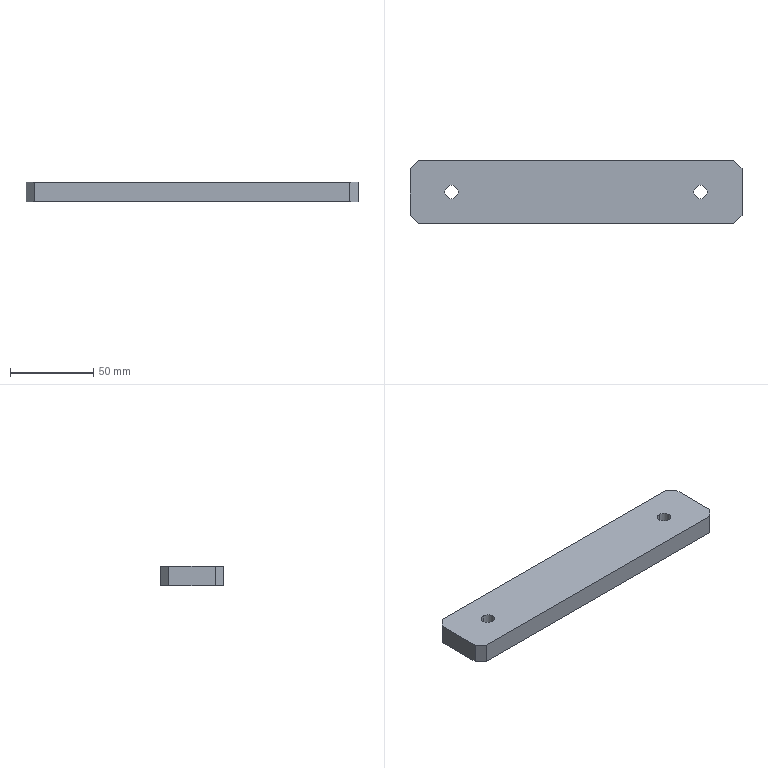Part | STEP file | [13] | 1 solid | 14 faces | box 200 x 38 x 12 mm | volume 89394 mm3 | plane 10 | cylinder 4 | commonest cylinder face diameters 8 x4
STEP:
#1=CARTESIAN_POINT('',(0.,0.,0.));
#2=DIRECTION('',(0.,0.,1.));
#3=DIRECTION('',(1.,0.,0.));
#4=AXIS2_PLACEMENT_3D('',#1,#2,#3);
#5=CARTESIAN_POINT('',(25.,23.,-3.));
#6=VERTEX_POINT('',#5);
#7=CARTESIAN_POINT('',(25.,23.,9.));
#8=VERTEX_POINT('',#7);
#9=CARTESIAN_POINT('',(25.,23.,-3.));
#10=DIRECTION('',(0.,0.,1.));
#11=VECTOR('',#10,1.);
#12=LINE('',#9,#11);
#13=CARTESIAN_POINT('',(25.,19.,-3.));
#14=DIRECTION('',(0.,0.,1.));
#15=DIRECTION('',(0.,1.,0.));
#16=AXIS2_PLACEMENT_3D('',#13,#14,#15);
#17=CYLINDRICAL_SURFACE('',#16,4.);
#18=CARTESIAN_POINT('',(6.283,0.));
#19=DIRECTION('',(0.,1.));
#20=VECTOR('',#19,1.);
#21=LINE('',#18,#20);
#22=(GEOMETRIC_REPRESENTATION_CONTEXT(2)PARAMETRIC_REPRESENTATION_CONTEXT()REPRESENTATION_CONTEXT('',''));
#23=DEFINITIONAL_REPRESENTATION('',(#21),#22);
#24=PCURVE('',#17,#23);
#25=CARTESIAN_POINT('',(25.,19.,-3.));
#26=DIRECTION('',(0.,0.,1.));
#27=DIRECTION('',(0.,1.,0.));
#28=AXIS2_PLACEMENT_3D('',#25,#26,#27);
#29=CYLINDRICAL_SURFACE('',#28,4.);
#30=CARTESIAN_POINT('',(0.,0.));
#31=DIRECTION('',(0.,1.));
#32=VECTOR('',#31,1.);
#33=LINE('',#30,#32);
#34=(GEOMETRIC_REPRESENTATION_CONTEXT(2)PARAMETRIC_REPRESENTATION_CONTEXT()REPRESENTATION_CONTEXT('',''));
#35=DEFINITIONAL_REPRESENTATION('',(#33),#34);
#36=PCURVE('',#29,#35);
#37=SURFACE_CURVE('',#12,(#24,#36),.PCURVE_S1.);
#38=EDGE_CURVE('',#6,#8,#37,.T.);
#39=ORIENTED_EDGE('',*,*,#38,.T.);
#40=CARTESIAN_POINT('',(25.,15.,9.));
#41=VERTEX_POINT('',#40);
#42=CARTESIAN_POINT('',(25.,19.,9.));
#43=DIRECTION('',(0.,0.,-1.));
#44=DIRECTION('',(0.,-1.,0.));
#45=AXIS2_PLACEMENT_3D('',#42,#43,#44);
#46=CIRCLE('',#45,4.);
#47=CARTESIAN_POINT('',(9.425,12.));
#48=DIRECTION('',(-1.,0.));
#49=VECTOR('',#48,1.);
#50=LINE('',#47,#49);
#51=(GEOMETRIC_REPRESENTATION_CONTEXT(2)PARAMETRIC_REPRESENTATION_CONTEXT()REPRESENTATION_CONTEXT('',''));
#52=DEFINITIONAL_REPRESENTATION('',(#50),#51);
#53=PCURVE('',#17,#52);
#54=CARTESIAN_POINT('',(100.,19.,9.));
#55=DIRECTION('',(0.,0.,1.));
#56=DIRECTION('',(0.,1.,0.));
#57=AXIS2_PLACEMENT_3D('',#54,#55,#56);
#58=PLANE('',#57);
#59=CARTESIAN_POINT('',(-4.,75.));
#60=CARTESIAN_POINT('',(-4.,81.928));
#61=CARTESIAN_POINT('',(2.,78.464));
#62=CARTESIAN_POINT('',(8.,75.));
#63=CARTESIAN_POINT('',(2.,71.536));
#64=CARTESIAN_POINT('',(-4.,68.072));
#65=CARTESIAN_POINT('',(-4.,75.));
#66=(BOUNDED_CURVE()B_SPLINE_CURVE(2,(#59,#60,#61,#62,#63,#64,#65),.UNSPECIFIED.,.T.,.F.)B_SPLINE_CURVE_WITH_KNOTS((1,2,2,2,2,1),(-2.094,0.,2.094,4.189,6.283,8.378),.UNSPECIFIED.)CURVE()GEOMETRIC_REPRESENTATION_ITEM()RATIONAL_B_SPLINE_CURVE((1.,0.5,1.,0.5,1.,0.5,1.))REPRESENTATION_ITEM(''));
#67=(GEOMETRIC_REPRESENTATION_CONTEXT(2)PARAMETRIC_REPRESENTATION_CONTEXT()REPRESENTATION_CONTEXT('',''));
#68=DEFINITIONAL_REPRESENTATION('',(#66),#67);
#69=PCURVE('',#58,#68);
#70=SURFACE_CURVE('',#46,(#53,#69),.PCURVE_S1.);
#71=EDGE_CURVE('',#8,#41,#70,.T.);
#72=ORIENTED_EDGE('',*,*,#71,.T.);
#73=CARTESIAN_POINT('',(25.,15.,-3.));
#74=VERTEX_POINT('',#73);
#75=CARTESIAN_POINT('',(25.,15.,-3.));
#76=DIRECTION('',(0.,0.,1.));
#77=VECTOR('',#76,1.);
#78=LINE('',#75,#77);
#79=CARTESIAN_POINT('',(3.142,0.));
#80=DIRECTION('',(0.,1.));
#81=VECTOR('',#80,1.);
#82=LINE('',#79,#81);
#83=(GEOMETRIC_REPRESENTATION_CONTEXT(2)PARAMETRIC_REPRESENTATION_CONTEXT()REPRESENTATION_CONTEXT('',''));
#84=DEFINITIONAL_REPRESENTATION('',(#82),#83);
#85=PCURVE('',#17,#84);
#86=CARTESIAN_POINT('',(3.142,0.));
#87=DIRECTION('',(0.,1.));
#88=VECTOR('',#87,1.);
#89=LINE('',#86,#88);
#90=(GEOMETRIC_REPRESENTATION_CONTEXT(2)PARAMETRIC_REPRESENTATION_CONTEXT()REPRESENTATION_CONTEXT('',''));
#91=DEFINITIONAL_REPRESENTATION('',(#89),#90);
#92=PCURVE('',#29,#91);
#93=SURFACE_CURVE('',#78,(#85,#92),.PCURVE_S1.);
#94=EDGE_CURVE('',#74,#41,#93,.T.);
#95=ORIENTED_EDGE('',*,*,#94,.F.);
#96=CARTESIAN_POINT('',(25.,19.,-3.));
#97=DIRECTION('',(0.,0.,1.));
#98=DIRECTION('',(0.,1.,0.));
#99=AXIS2_PLACEMENT_3D('',#96,#97,#98);
#100=CIRCLE('',#99,4.);
#101=CARTESIAN_POINT('',(0.,0.));
#102=DIRECTION('',(1.,0.));
#103=VECTOR('',#102,1.);
#104=LINE('',#101,#103);
#105=(GEOMETRIC_REPRESENTATION_CONTEXT(2)PARAMETRIC_REPRESENTATION_CONTEXT()REPRESENTATION_CONTEXT('',''));
#106=DEFINITIONAL_REPRESENTATION('',(#104),#105);
#107=PCURVE('',#17,#106);
#108=CARTESIAN_POINT('',(100.,19.,-3.));
#109=DIRECTION('',(0.,0.,-1.));
#110=DIRECTION('',(0.,-1.,0.));
#111=AXIS2_PLACEMENT_3D('',#108,#109,#110);
#112=PLANE('',#111);
#113=CARTESIAN_POINT('',(-4.,75.));
#114=CARTESIAN_POINT('',(-4.,81.928));
#115=CARTESIAN_POINT('',(2.,78.464));
#116=CARTESIAN_POINT('',(8.,75.));
#117=CARTESIAN_POINT('',(2.,71.536));
#118=CARTESIAN_POINT('',(-4.,68.072));
#119=CARTESIAN_POINT('',(-4.,75.));
#120=(BOUNDED_CURVE()B_SPLINE_CURVE(2,(#113,#114,#115,#116,#117,#118,#119),.UNSPECIFIED.,.T.,.F.)B_SPLINE_CURVE_WITH_KNOTS((1,2,2,2,2,1),(-2.094,0.,2.094,4.189,6.283,8.378),.UNSPECIFIED.)CURVE()GEOMETRIC_REPRESENTATION_ITEM()RATIONAL_B_SPLINE_CURVE((1.,0.5,1.,0.5,1.,0.5,1.))REPRESENTATION_ITEM(''));
#121=(GEOMETRIC_REPRESENTATION_CONTEXT(2)PARAMETRIC_REPRESENTATION_CONTEXT()REPRESENTATION_CONTEXT('',''));
#122=DEFINITIONAL_REPRESENTATION('',(#120),#121);
#123=PCURVE('',#112,#122);
#124=SURFACE_CURVE('',#100,(#107,#123),.PCURVE_S1.);
#125=EDGE_CURVE('',#74,#6,#124,.T.);
#126=ORIENTED_EDGE('',*,*,#125,.T.);
#127=EDGE_LOOP('',(#39,#72,#95,#126));
#128=FACE_BOUND('',#127,.F.);
#129=ADVANCED_FACE('',(#128),#17,.F.);
#130=CARTESIAN_POINT('',(175.,23.,-3.));
#131=VERTEX_POINT('',#130);
#132=CARTESIAN_POINT('',(175.,23.,9.));
#133=VERTEX_POINT('',#132);
#134=CARTESIAN_POINT('',(175.,23.,-3.));
#135=DIRECTION('',(0.,0.,1.));
#136=VECTOR('',#135,1.);
#137=LINE('',#134,#136);
#138=CARTESIAN_POINT('',(175.,19.,-3.));
#139=DIRECTION('',(0.,0.,1.));
#140=DIRECTION('',(0.,1.,0.));
#141=AXIS2_PLACEMENT_3D('',#138,#139,#140);
#142=CYLINDRICAL_SURFACE('',#141,4.);
#143=CARTESIAN_POINT('',(6.283,0.));
#144=DIRECTION('',(0.,1.));
#145=VECTOR('',#144,1.);
#146=LINE('',#143,#145);
#147=(GEOMETRIC_REPRESENTATION_CONTEXT(2)PARAMETRIC_REPRESENTATION_CONTEXT()REPRESENTATION_CONTEXT('',''));
#148=DEFINITIONAL_REPRESENTATION('',(#146),#147);
#149=PCURVE('',#142,#148);
#150=CARTESIAN_POINT('',(175.,19.,-3.));
#151=DIRECTION('',(0.,0.,1.));
#152=DIRECTION('',(0.,1.,0.));
#153=AXIS2_PLACEMENT_3D('',#150,#151,#152);
#154=CYLINDRICAL_SURFACE('',#153,4.);
#155=CARTESIAN_POINT('',(0.,0.));
#156=DIRECTION('',(0.,1.));
#157=VECTOR('',#156,1.);
#158=LINE('',#155,#157);
#159=(GEOMETRIC_REPRESENTATION_CONTEXT(2)PARAMETRIC_REPRESENTATION_CONTEXT()REPRESENTATION_CONTEXT('',''));
#160=DEFINITIONAL_REPRESENTATION('',(#158),#159);
#161=PCURVE('',#154,#160);
#162=SURFACE_CURVE('',#137,(#149,#161),.PCURVE_S1.);
#163=EDGE_CURVE('',#131,#133,#162,.T.);
#164=ORIENTED_EDGE('',*,*,#163,.T.);
#165=CARTESIAN_POINT('',(175.,15.,9.));
#166=VERTEX_POINT('',#165);
#167=CARTESIAN_POINT('',(175.,19.,9.));
#168=DIRECTION('',(0.,0.,-1.));
#169=DIRECTION('',(0.,-1.,0.));
#170=AXIS2_PLACEMENT_3D('',#167,#168,#169);
#171=CIRCLE('',#170,4.);
#172=CARTESIAN_POINT('',(9.425,12.));
#173=DIRECTION('',(-1.,0.));
#174=VECTOR('',#173,1.);
#175=LINE('',#172,#174);
#176=(GEOMETRIC_REPRESENTATION_CONTEXT(2)PARAMETRIC_REPRESENTATION_CONTEXT()REPRESENTATION_CONTEXT('',''));
#177=DEFINITIONAL_REPRESENTATION('',(#175),#176);
#178=PCURVE('',#142,#177);
#179=CARTESIAN_POINT('',(-4.,-75.));
#180=CARTESIAN_POINT('',(-4.,-68.072));
#181=CARTESIAN_POINT('',(2.,-71.536));
#182=CARTESIAN_POINT('',(8.,-75.));
#183=CARTESIAN_POINT('',(2.,-78.464));
#184=CARTESIAN_POINT('',(-4.,-81.928));
#185=CARTESIAN_POINT('',(-4.,-75.));
#186=(BOUNDED_CURVE()B_SPLINE_CURVE(2,(#179,#180,#181,#182,#183,#184,#185),.UNSPECIFIED.,.T.,.F.)B_SPLINE_CURVE_WITH_KNOTS((1,2,2,2,2,1),(-2.094,0.,2.094,4.189,6.283,8.378),.UNSPECIFIED.)CURVE()GEOMETRIC_REPRESENTATION_ITEM()RATIONAL_B_SPLINE_CURVE((1.,0.5,1.,0.5,1.,0.5,1.))REPRESENTATION_ITEM(''));
#187=(GEOMETRIC_REPRESENTATION_CONTEXT(2)PARAMETRIC_REPRESENTATION_CONTEXT()REPRESENTATION_CONTEXT('',''));
#188=DEFINITIONAL_REPRESENTATION('',(#186),#187);
#189=PCURVE('',#58,#188);
#190=SURFACE_CURVE('',#171,(#178,#189),.PCURVE_S1.);
#191=EDGE_CURVE('',#133,#166,#190,.T.);
#192=ORIENTED_EDGE('',*,*,#191,.T.);
#193=CARTESIAN_POINT('',(175.,15.,-3.));
#194=VERTEX_POINT('',#193);
#195=CARTESIAN_POINT('',(175.,15.,-3.));
#196=DIRECTION('',(0.,0.,1.));
#197=VECTOR('',#196,1.);
#198=LINE('',#195,#197);
#199=CARTESIAN_POINT('',(3.142,0.));
#200=DIRECTION('',(0.,1.));
#201=VECTOR('',#200,1.);
#202=LINE('',#199,#201);
#203=(GEOMETRIC_REPRESENTATION_CONTEXT(2)PARAMETRIC_REPRESENTATION_CONTEXT()REPRESENTATION_CONTEXT('',''));
#204=DEFINITIONAL_REPRESENTATION('',(#202),#203);
#205=PCURVE('',#142,#204);
#206=CARTESIAN_POINT('',(3.142,0.));
#207=DIRECTION('',(0.,1.));
#208=VECTOR('',#207,1.);
#209=LINE('',#206,#208);
#210=(GEOMETRIC_REPRESENTATION_CONTEXT(2)PARAMETRIC_REPRESENTATION_CONTEXT()REPRESENTATION_CONTEXT('',''));
#211=DEFINITIONAL_REPRESENTATION('',(#209),#210);
#212=PCURVE('',#154,#211);
#213=SURFACE_CURVE('',#198,(#205,#212),.PCURVE_S1.);
#214=EDGE_CURVE('',#194,#166,#213,.T.);
#215=ORIENTED_EDGE('',*,*,#214,.F.);
#216=CARTESIAN_POINT('',(175.,19.,-3.));
#217=DIRECTION('',(0.,0.,1.));
#218=DIRECTION('',(0.,1.,0.));
#219=AXIS2_PLACEMENT_3D('',#216,#217,#218);
#220=CIRCLE('',#219,4.);
#221=CARTESIAN_POINT('',(0.,0.));
#222=DIRECTION('',(1.,0.));
#223=VECTOR('',#222,1.);
#224=LINE('',#221,#223);
#225=(GEOMETRIC_REPRESENTATION_CONTEXT(2)PARAMETRIC_REPRESENTATION_CONTEXT()REPRESENTATION_CONTEXT('',''));
#226=DEFINITIONAL_REPRESENTATION('',(#224),#225);
#227=PCURVE('',#142,#226);
#228=CARTESIAN_POINT('',(-4.,-75.));
#229=CARTESIAN_POINT('',(-4.,-68.072));
#230=CARTESIAN_POINT('',(2.,-71.536));
#231=CARTESIAN_POINT('',(8.,-75.));
#232=CARTESIAN_POINT('',(2.,-78.464));
#233=CARTESIAN_POINT('',(-4.,-81.928));
#234=CARTESIAN_POINT('',(-4.,-75.));
#235=(BOUNDED_CURVE()B_SPLINE_CURVE(2,(#228,#229,#230,#231,#232,#233,#234),.UNSPECIFIED.,.T.,.F.)B_SPLINE_CURVE_WITH_KNOTS((1,2,2,2,2,1),(-2.094,0.,2.094,4.189,6.283,8.378),.UNSPECIFIED.)CURVE()GEOMETRIC_REPRESENTATION_ITEM()RATIONAL_B_SPLINE_CURVE((1.,0.5,1.,0.5,1.,0.5,1.))REPRESENTATION_ITEM(''));
#236=(GEOMETRIC_REPRESENTATION_CONTEXT(2)PARAMETRIC_REPRESENTATION_CONTEXT()REPRESENTATION_CONTEXT('',''));
#237=DEFINITIONAL_REPRESENTATION('',(#235),#236);
#238=PCURVE('',#112,#237);
#239=SURFACE_CURVE('',#220,(#227,#238),.PCURVE_S1.);
#240=EDGE_CURVE('',#194,#131,#239,.T.);
#241=ORIENTED_EDGE('',*,*,#240,.T.);
#242=EDGE_LOOP('',(#164,#192,#215,#241));
#243=FACE_BOUND('',#242,.F.);
#244=ADVANCED_FACE('',(#243),#142,.F.);
#245=CARTESIAN_POINT('',(25.,19.,-3.));
#246=DIRECTION('',(0.,0.,1.));
#247=DIRECTION('',(0.,1.,0.));
#248=AXIS2_PLACEMENT_3D('',#245,#246,#247);
#249=CIRCLE('',#248,4.);
#250=CARTESIAN_POINT('',(-4.,75.));
#251=CARTESIAN_POINT('',(-4.,81.928));
#252=CARTESIAN_POINT('',(2.,78.464));
#253=CARTESIAN_POINT('',(8.,75.));
#254=CARTESIAN_POINT('',(2.,71.536));
#255=CARTESIAN_POINT('',(-4.,68.072));
#256=CARTESIAN_POINT('',(-4.,75.));
#257=(BOUNDED_CURVE()B_SPLINE_CURVE(2,(#250,#251,#252,#253,#254,#255,#256),.UNSPECIFIED.,.T.,.F.)B_SPLINE_CURVE_WITH_KNOTS((1,2,2,2,2,1),(-2.094,0.,2.094,4.189,6.283,8.378),.UNSPECIFIED.)CURVE()GEOMETRIC_REPRESENTATION_ITEM()RATIONAL_B_SPLINE_CURVE((1.,0.5,1.,0.5,1.,0.5,1.))REPRESENTATION_ITEM(''));
#258=(GEOMETRIC_REPRESENTATION_CONTEXT(2)PARAMETRIC_REPRESENTATION_CONTEXT()REPRESENTATION_CONTEXT('',''));
#259=DEFINITIONAL_REPRESENTATION('',(#257),#258);
#260=PCURVE('',#112,#259);
#261=CARTESIAN_POINT('',(0.,0.));
#262=DIRECTION('',(1.,0.));
#263=VECTOR('',#262,1.);
#264=LINE('',#261,#263);
#265=(GEOMETRIC_REPRESENTATION_CONTEXT(2)PARAMETRIC_REPRESENTATION_CONTEXT()REPRESENTATION_CONTEXT('',''));
#266=DEFINITIONAL_REPRESENTATION('',(#264),#265);
#267=PCURVE('',#29,#266);
#268=SURFACE_CURVE('',#249,(#260,#267),.PCURVE_S1.);
#269=EDGE_CURVE('',#6,#74,#268,.T.);
#270=ORIENTED_EDGE('',*,*,#269,.T.);
#271=ORIENTED_EDGE('',*,*,#125,.T.);
#272=EDGE_LOOP('',(#270,#271));
#273=FACE_BOUND('',#272,.T.);
#274=CARTESIAN_POINT('',(175.,19.,-3.));
#275=DIRECTION('',(0.,0.,1.));
#276=DIRECTION('',(0.,1.,0.));
#277=AXIS2_PLACEMENT_3D('',#274,#275,#276);
#278=CIRCLE('',#277,4.);
#279=CARTESIAN_POINT('',(-4.,-75.));
#280=CARTESIAN_POINT('',(-4.,-68.072));
#281=CARTESIAN_POINT('',(2.,-71.536));
#282=CARTESIAN_POINT('',(8.,-75.));
#283=CARTESIAN_POINT('',(2.,-78.464));
#284=CARTESIAN_POINT('',(-4.,-81.928));
#285=CARTESIAN_POINT('',(-4.,-75.));
#286=(BOUNDED_CURVE()B_SPLINE_CURVE(2,(#279,#280,#281,#282,#283,#284,#285),.UNSPECIFIED.,.T.,.F.)B_SPLINE_CURVE_WITH_KNOTS((1,2,2,2,2,1),(-2.094,0.,2.094,4.189,6.283,8.378),.UNSPECIFIED.)CURVE()GEOMETRIC_REPRESENTATION_ITEM()RATIONAL_B_SPLINE_CURVE((1.,0.5,1.,0.5,1.,0.5,1.))REPRESENTATION_ITEM(''));
#287=(GEOMETRIC_REPRESENTATION_CONTEXT(2)PARAMETRIC_REPRESENTATION_CONTEXT()REPRESENTATION_CONTEXT('',''));
#288=DEFINITIONAL_REPRESENTATION('',(#286),#287);
#289=PCURVE('',#112,#288);
#290=CARTESIAN_POINT('',(0.,0.));
#291=DIRECTION('',(1.,0.));
#292=VECTOR('',#291,1.);
#293=LINE('',#290,#292);
#294=(GEOMETRIC_REPRESENTATION_CONTEXT(2)PARAMETRIC_REPRESENTATION_CONTEXT()REPRESENTATION_CONTEXT('',''));
#295=DEFINITIONAL_REPRESENTATION('',(#293),#294);
#296=PCURVE('',#154,#295);
#297=SURFACE_CURVE('',#278,(#289,#296),.PCURVE_S1.);
#298=EDGE_CURVE('',#131,#194,#297,.T.);
#299=ORIENTED_EDGE('',*,*,#298,.T.);
#300=ORIENTED_EDGE('',*,*,#240,.T.);
#301=EDGE_LOOP('',(#299,#300));
#302=FACE_BOUND('',#301,.T.);
#303=CARTESIAN_POINT('',(5.,0.,-3.));
#304=VERTEX_POINT('',#303);
#305=CARTESIAN_POINT('',(195.,0.,-3.));
#306=VERTEX_POINT('',#305);
#307=CARTESIAN_POINT('',(100.,0.,-3.));
#308=DIRECTION('',(1.,0.,0.));
#309=VECTOR('',#308,1.);
#310=LINE('',#307,#309);
#311=CARTESIAN_POINT('',(19.,0.));
#312=DIRECTION('',(0.,-1.));
#313=VECTOR('',#312,1.);
#314=LINE('',#311,#313);
#315=(GEOMETRIC_REPRESENTATION_CONTEXT(2)PARAMETRIC_REPRESENTATION_CONTEXT()REPRESENTATION_CONTEXT('',''));
#316=DEFINITIONAL_REPRESENTATION('',(#314),#315);
#317=PCURVE('',#112,#316);
#318=CARTESIAN_POINT('',(100.,0.,9.));
#319=DIRECTION('',(0.,-1.,0.));
#320=DIRECTION('',(0.,0.,1.));
#321=AXIS2_PLACEMENT_3D('',#318,#319,#320);
#322=PLANE('',#321);
#323=CARTESIAN_POINT('',(-12.,0.));
#324=DIRECTION('',(0.,-1.));
#325=VECTOR('',#324,1.);
#326=LINE('',#323,#325);
#327=(GEOMETRIC_REPRESENTATION_CONTEXT(2)PARAMETRIC_REPRESENTATION_CONTEXT()REPRESENTATION_CONTEXT('',''));
#328=DEFINITIONAL_REPRESENTATION('',(#326),#327);
#329=PCURVE('',#322,#328);
#330=SURFACE_CURVE('',#310,(#317,#329),.PCURVE_S1.);
#331=EDGE_CURVE('',#304,#306,#330,.T.);
#332=ORIENTED_EDGE('',*,*,#331,.F.);
#333=CARTESIAN_POINT('',(0.,5.,-3.));
#334=VERTEX_POINT('',#333);
#335=CARTESIAN_POINT('',(43.,-38.,-3.));
#336=DIRECTION('',(-0.7071,0.7071,0.));
#337=VECTOR('',#336,1.);
#338=LINE('',#335,#337);
#339=CARTESIAN_POINT('',(57.,57.));
#340=DIRECTION('',(-0.7071,0.7071));
#341=VECTOR('',#340,1.);
#342=LINE('',#339,#341);
#343=(GEOMETRIC_REPRESENTATION_CONTEXT(2)PARAMETRIC_REPRESENTATION_CONTEXT()REPRESENTATION_CONTEXT('',''));
#344=DEFINITIONAL_REPRESENTATION('',(#342),#343);
#345=PCURVE('',#112,#344);
#346=CARTESIAN_POINT('',(5.,0.,9.));
#347=DIRECTION('',(0.7071,0.7071,0.));
#348=DIRECTION('',(0.,0.,-1.));
#349=AXIS2_PLACEMENT_3D('',#346,#347,#348);
#350=PLANE('',#349);
#351=CARTESIAN_POINT('',(12.,-53.74));
#352=DIRECTION('',(0.,1.));
#353=VECTOR('',#352,1.);
#354=LINE('',#351,#353);
#355=(GEOMETRIC_REPRESENTATION_CONTEXT(2)PARAMETRIC_REPRESENTATION_CONTEXT()REPRESENTATION_CONTEXT('',''));
#356=DEFINITIONAL_REPRESENTATION('',(#354),#355);
#357=PCURVE('',#350,#356);
#358=SURFACE_CURVE('',#338,(#345,#357),.PCURVE_S1.);
#359=EDGE_CURVE('',#304,#334,#358,.T.);
#360=ORIENTED_EDGE('',*,*,#359,.T.);
#361=CARTESIAN_POINT('',(0.,33.,-3.));
#362=VERTEX_POINT('',#361);
#363=CARTESIAN_POINT('',(0.,19.,-3.));
#364=DIRECTION('',(0.,-1.,0.));
#365=VECTOR('',#364,1.);
#366=LINE('',#363,#365);
#367=CARTESIAN_POINT('',(0.,100.));
#368=DIRECTION('',(1.,0.));
#369=VECTOR('',#368,1.);
#370=LINE('',#367,#369);
#371=(GEOMETRIC_REPRESENTATION_CONTEXT(2)PARAMETRIC_REPRESENTATION_CONTEXT()REPRESENTATION_CONTEXT('',''));
#372=DEFINITIONAL_REPRESENTATION('',(#370),#371);
#373=PCURVE('',#112,#372);
#374=CARTESIAN_POINT('',(0.,19.,9.));
#375=DIRECTION('',(-1.,0.,0.));
#376=DIRECTION('',(0.,0.,-1.));
#377=AXIS2_PLACEMENT_3D('',#374,#375,#376);
#378=PLANE('',#377);
#379=CARTESIAN_POINT('',(12.,0.));
#380=DIRECTION('',(0.,1.));
#381=VECTOR('',#380,1.);
#382=LINE('',#379,#381);
#383=(GEOMETRIC_REPRESENTATION_CONTEXT(2)PARAMETRIC_REPRESENTATION_CONTEXT()REPRESENTATION_CONTEXT('',''));
#384=DEFINITIONAL_REPRESENTATION('',(#382),#383);
#385=PCURVE('',#378,#384);
#386=SURFACE_CURVE('',#366,(#373,#385),.PCURVE_S1.);
#387=EDGE_CURVE('',#362,#334,#386,.T.);
#388=ORIENTED_EDGE('',*,*,#387,.F.);
#389=CARTESIAN_POINT('',(5.,38.,-3.));
#390=VERTEX_POINT('',#389);
#391=CARTESIAN_POINT('',(43.,76.,-3.));
#392=DIRECTION('',(0.7071,0.7071,0.));
#393=VECTOR('',#392,1.);
#394=LINE('',#391,#393);
#395=CARTESIAN_POINT('',(-57.,57.));
#396=DIRECTION('',(-0.7071,-0.7071));
#397=VECTOR('',#396,1.);
#398=LINE('',#395,#397);
#399=(GEOMETRIC_REPRESENTATION_CONTEXT(2)PARAMETRIC_REPRESENTATION_CONTEXT()REPRESENTATION_CONTEXT('',''));
#400=DEFINITIONAL_REPRESENTATION('',(#398),#399);
#401=PCURVE('',#112,#400);
#402=CARTESIAN_POINT('',(0.,33.,9.));
#403=DIRECTION('',(0.7071,-0.7071,0.));
#404=DIRECTION('',(0.,0.,-1.));
#405=AXIS2_PLACEMENT_3D('',#402,#403,#404);
#406=PLANE('',#405);
#407=CARTESIAN_POINT('',(12.,60.811));
#408=DIRECTION('',(0.,1.));
#409=VECTOR('',#408,1.);
#410=LINE('',#407,#409);
#411=(GEOMETRIC_REPRESENTATION_CONTEXT(2)PARAMETRIC_REPRESENTATION_CONTEXT()REPRESENTATION_CONTEXT('',''));
#412=DEFINITIONAL_REPRESENTATION('',(#410),#411);
#413=PCURVE('',#406,#412);
#414=SURFACE_CURVE('',#394,(#401,#413),.PCURVE_S1.);
#415=EDGE_CURVE('',#362,#390,#414,.T.);
#416=ORIENTED_EDGE('',*,*,#415,.T.);
#417=CARTESIAN_POINT('',(195.,38.,-3.));
#418=VERTEX_POINT('',#417);
#419=CARTESIAN_POINT('',(100.,38.,-3.));
#420=DIRECTION('',(-1.,0.,0.));
#421=VECTOR('',#420,1.);
#422=LINE('',#419,#421);
#423=CARTESIAN_POINT('',(-19.,0.));
#424=DIRECTION('',(0.,1.));
#425=VECTOR('',#424,1.);
#426=LINE('',#423,#425);
#427=(GEOMETRIC_REPRESENTATION_CONTEXT(2)PARAMETRIC_REPRESENTATION_CONTEXT()REPRESENTATION_CONTEXT('',''));
#428=DEFINITIONAL_REPRESENTATION('',(#426),#427);
#429=PCURVE('',#112,#428);
#430=CARTESIAN_POINT('',(100.,38.,9.));
#431=DIRECTION('',(0.,1.,0.));
#432=DIRECTION('',(0.,0.,-1.));
#433=AXIS2_PLACEMENT_3D('',#430,#431,#432);
#434=PLANE('',#433);
#435=CARTESIAN_POINT('',(12.,0.));
#436=DIRECTION('',(0.,1.));
#437=VECTOR('',#436,1.);
#438=LINE('',#435,#437);
#439=(GEOMETRIC_REPRESENTATION_CONTEXT(2)PARAMETRIC_REPRESENTATION_CONTEXT()REPRESENTATION_CONTEXT('',''));
#440=DEFINITIONAL_REPRESENTATION('',(#438),#439);
#441=PCURVE('',#434,#440);
#442=SURFACE_CURVE('',#422,(#429,#441),.PCURVE_S1.);
#443=EDGE_CURVE('',#418,#390,#442,.T.);
#444=ORIENTED_EDGE('',*,*,#443,.F.);
#445=CARTESIAN_POINT('',(200.,33.,-3.));
#446=VERTEX_POINT('',#445);
#447=CARTESIAN_POINT('',(157.,76.,-3.));
#448=DIRECTION('',(0.7071,-0.7071,0.));
#449=VECTOR('',#448,1.);
#450=LINE('',#447,#449);
#451=CARTESIAN_POINT('',(-57.,-57.));
#452=DIRECTION('',(0.7071,-0.7071));
#453=VECTOR('',#452,1.);
#454=LINE('',#451,#453);
#455=(GEOMETRIC_REPRESENTATION_CONTEXT(2)PARAMETRIC_REPRESENTATION_CONTEXT()REPRESENTATION_CONTEXT('',''));
#456=DEFINITIONAL_REPRESENTATION('',(#454),#455);
#457=PCURVE('',#112,#456);
#458=CARTESIAN_POINT('',(195.,38.,9.));
#459=DIRECTION('',(-0.7071,-0.7071,0.));
#460=DIRECTION('',(0.,0.,-1.));
#461=AXIS2_PLACEMENT_3D('',#458,#459,#460);
#462=PLANE('',#461);
#463=CARTESIAN_POINT('',(12.,-53.74));
#464=DIRECTION('',(0.,1.));
#465=VECTOR('',#464,1.);
#466=LINE('',#463,#465);
#467=(GEOMETRIC_REPRESENTATION_CONTEXT(2)PARAMETRIC_REPRESENTATION_CONTEXT()REPRESENTATION_CONTEXT('',''));
#468=DEFINITIONAL_REPRESENTATION('',(#466),#467);
#469=PCURVE('',#462,#468);
#470=SURFACE_CURVE('',#450,(#457,#469),.PCURVE_S1.);
#471=EDGE_CURVE('',#418,#446,#470,.T.);
#472=ORIENTED_EDGE('',*,*,#471,.T.);
#473=CARTESIAN_POINT('',(200.,5.,-3.));
#474=VERTEX_POINT('',#473);
#475=CARTESIAN_POINT('',(200.,19.,-3.));
#476=DIRECTION('',(0.,1.,0.));
#477=VECTOR('',#476,1.);
#478=LINE('',#475,#477);
#479=CARTESIAN_POINT('',(0.,-100.));
#480=DIRECTION('',(-1.,0.));
#481=VECTOR('',#480,1.);
#482=LINE('',#479,#481);
#483=(GEOMETRIC_REPRESENTATION_CONTEXT(2)PARAMETRIC_REPRESENTATION_CONTEXT()REPRESENTATION_CONTEXT('',''));
#484=DEFINITIONAL_REPRESENTATION('',(#482),#483);
#485=PCURVE('',#112,#484);
#486=CARTESIAN_POINT('',(200.,19.,9.));
#487=DIRECTION('',(1.,0.,0.));
#488=DIRECTION('',(0.,0.,1.));
#489=AXIS2_PLACEMENT_3D('',#486,#487,#488);
#490=PLANE('',#489);
#491=CARTESIAN_POINT('',(-12.,0.));
#492=DIRECTION('',(0.,-1.));
#493=VECTOR('',#492,1.);
#494=LINE('',#491,#493);
#495=(GEOMETRIC_REPRESENTATION_CONTEXT(2)PARAMETRIC_REPRESENTATION_CONTEXT()REPRESENTATION_CONTEXT('',''));
#496=DEFINITIONAL_REPRESENTATION('',(#494),#495);
#497=PCURVE('',#490,#496);
#498=SURFACE_CURVE('',#478,(#485,#497),.PCURVE_S1.);
#499=EDGE_CURVE('',#474,#446,#498,.T.);
#500=ORIENTED_EDGE('',*,*,#499,.F.);
#501=CARTESIAN_POINT('',(157.,-38.,-3.));
#502=DIRECTION('',(-0.7071,-0.7071,0.));
#503=VECTOR('',#502,1.);
#504=LINE('',#501,#503);
#505=CARTESIAN_POINT('',(57.,-57.));
#506=DIRECTION('',(0.7071,0.7071));
#507=VECTOR('',#506,1.);
#508=LINE('',#505,#507);
#509=(GEOMETRIC_REPRESENTATION_CONTEXT(2)PARAMETRIC_REPRESENTATION_CONTEXT()REPRESENTATION_CONTEXT('',''));
#510=DEFINITIONAL_REPRESENTATION('',(#508),#509);
#511=PCURVE('',#112,#510);
#512=CARTESIAN_POINT('',(200.,5.,9.));
#513=DIRECTION('',(-0.7071,0.7071,0.));
#514=DIRECTION('',(0.,0.,-1.));
#515=AXIS2_PLACEMENT_3D('',#512,#513,#514);
#516=PLANE('',#515);
#517=CARTESIAN_POINT('',(12.,60.811));
#518=DIRECTION('',(0.,1.));
#519=VECTOR('',#518,1.);
#520=LINE('',#517,#519);
#521=(GEOMETRIC_REPRESENTATION_CONTEXT(2)PARAMETRIC_REPRESENTATION_CONTEXT()REPRESENTATION_CONTEXT('',''));
#522=DEFINITIONAL_REPRESENTATION('',(#520),#521);
#523=PCURVE('',#516,#522);
#524=SURFACE_CURVE('',#504,(#511,#523),.PCURVE_S1.);
#525=EDGE_CURVE('',#474,#306,#524,.T.);
#526=ORIENTED_EDGE('',*,*,#525,.T.);
#527=EDGE_LOOP('',(#332,#360,#388,#416,#444,#472,#500,#526));
#528=FACE_BOUND('',#527,.T.);
#529=ADVANCED_FACE('',(#273,#302,#528),#112,.T.);
#530=CARTESIAN_POINT('',(200.,33.,9.));
#531=VERTEX_POINT('',#530);
#532=CARTESIAN_POINT('',(200.,5.,9.));
#533=VERTEX_POINT('',#532);
#534=CARTESIAN_POINT('',(200.,19.,9.));
#535=DIRECTION('',(0.,-1.,0.));
#536=VECTOR('',#535,1.);
#537=LINE('',#534,#536);
#538=CARTESIAN_POINT('',(0.,0.));
#539=DIRECTION('',(0.,1.));
#540=VECTOR('',#539,1.);
#541=LINE('',#538,#540);
#542=(GEOMETRIC_REPRESENTATION_CONTEXT(2)PARAMETRIC_REPRESENTATION_CONTEXT()REPRESENTATION_CONTEXT('',''));
#543=DEFINITIONAL_REPRESENTATION('',(#541),#542);
#544=PCURVE('',#490,#543);
#545=CARTESIAN_POINT('',(0.,-100.));
#546=DIRECTION('',(-1.,0.));
#547=VECTOR('',#546,1.);
#548=LINE('',#545,#547);
#549=(GEOMETRIC_REPRESENTATION_CONTEXT(2)PARAMETRIC_REPRESENTATION_CONTEXT()REPRESENTATION_CONTEXT('',''));
#550=DEFINITIONAL_REPRESENTATION('',(#548),#549);
#551=PCURVE('',#58,#550);
#552=SURFACE_CURVE('',#537,(#544,#551),.PCURVE_S1.);
#553=EDGE_CURVE('',#531,#533,#552,.T.);
#554=ORIENTED_EDGE('',*,*,#553,.T.);
#555=CARTESIAN_POINT('',(200.,5.,9.));
#556=DIRECTION('',(0.,0.,-1.));
#557=VECTOR('',#556,1.);
#558=LINE('',#555,#557);
#559=CARTESIAN_POINT('',(0.,14.));
#560=DIRECTION('',(-1.,0.));
#561=VECTOR('',#560,1.);
#562=LINE('',#559,#561);
#563=(GEOMETRIC_REPRESENTATION_CONTEXT(2)PARAMETRIC_REPRESENTATION_CONTEXT()REPRESENTATION_CONTEXT('',''));
#564=DEFINITIONAL_REPRESENTATION('',(#562),#563);
#565=PCURVE('',#490,#564);
#566=CARTESIAN_POINT('',(0.,0.));
#567=DIRECTION('',(1.,0.));
#568=VECTOR('',#567,1.);
#569=LINE('',#566,#568);
#570=(GEOMETRIC_REPRESENTATION_CONTEXT(2)PARAMETRIC_REPRESENTATION_CONTEXT()REPRESENTATION_CONTEXT('',''));
#571=DEFINITIONAL_REPRESENTATION('',(#569),#570);
#572=PCURVE('',#516,#571);
#573=SURFACE_CURVE('',#558,(#565,#572),.PCURVE_S1.);
#574=EDGE_CURVE('',#533,#474,#573,.T.);
#575=ORIENTED_EDGE('',*,*,#574,.T.);
#576=ORIENTED_EDGE('',*,*,#499,.T.);
#577=CARTESIAN_POINT('',(200.,33.,9.));
#578=DIRECTION('',(0.,0.,1.));
#579=VECTOR('',#578,1.);
#580=LINE('',#577,#579);
#581=CARTESIAN_POINT('',(0.,-14.));
#582=DIRECTION('',(1.,0.));
#583=VECTOR('',#582,1.);
#584=LINE('',#581,#583);
#585=(GEOMETRIC_REPRESENTATION_CONTEXT(2)PARAMETRIC_REPRESENTATION_CONTEXT()REPRESENTATION_CONTEXT('',''));
#586=DEFINITIONAL_REPRESENTATION('',(#584),#585);
#587=PCURVE('',#490,#586);
#588=CARTESIAN_POINT('',(0.,7.071));
#589=DIRECTION('',(-1.,0.));
#590=VECTOR('',#589,1.);
#591=LINE('',#588,#590);
#592=(GEOMETRIC_REPRESENTATION_CONTEXT(2)PARAMETRIC_REPRESENTATION_CONTEXT()REPRESENTATION_CONTEXT('',''));
#593=DEFINITIONAL_REPRESENTATION('',(#591),#592);
#594=PCURVE('',#462,#593);
#595=SURFACE_CURVE('',#580,(#587,#594),.PCURVE_S1.);
#596=EDGE_CURVE('',#446,#531,#595,.T.);
#597=ORIENTED_EDGE('',*,*,#596,.T.);
#598=EDGE_LOOP('',(#554,#575,#576,#597));
#599=FACE_BOUND('',#598,.T.);
#600=ADVANCED_FACE('',(#599),#490,.T.);
#601=ORIENTED_EDGE('',*,*,#443,.T.);
#602=CARTESIAN_POINT('',(5.,38.,9.));
#603=VERTEX_POINT('',#602);
#604=CARTESIAN_POINT('',(5.,38.,9.));
#605=DIRECTION('',(0.,0.,1.));
#606=VECTOR('',#605,1.);
#607=LINE('',#604,#606);
#608=CARTESIAN_POINT('',(0.,95.));
#609=DIRECTION('',(-1.,0.));
#610=VECTOR('',#609,1.);
#611=LINE('',#608,#610);
#612=(GEOMETRIC_REPRESENTATION_CONTEXT(2)PARAMETRIC_REPRESENTATION_CONTEXT()REPRESENTATION_CONTEXT('',''));
#613=DEFINITIONAL_REPRESENTATION('',(#611),#612);
#614=PCURVE('',#434,#613);
#615=CARTESIAN_POINT('',(0.,7.071));
#616=DIRECTION('',(-1.,0.));
#617=VECTOR('',#616,1.);
#618=LINE('',#615,#617);
#619=(GEOMETRIC_REPRESENTATION_CONTEXT(2)PARAMETRIC_REPRESENTATION_CONTEXT()REPRESENTATION_CONTEXT('',''));
#620=DEFINITIONAL_REPRESENTATION('',(#618),#619);
#621=PCURVE('',#406,#620);
#622=SURFACE_CURVE('',#607,(#614,#621),.PCURVE_S1.);
#623=EDGE_CURVE('',#390,#603,#622,.T.);
#624=ORIENTED_EDGE('',*,*,#623,.T.);
#625=CARTESIAN_POINT('',(195.,38.,9.));
#626=VERTEX_POINT('',#625);
#627=CARTESIAN_POINT('',(100.,38.,9.));
#628=DIRECTION('',(1.,0.,0.));
#629=VECTOR('',#628,1.);
#630=LINE('',#627,#629);
#631=CARTESIAN_POINT('',(0.,0.));
#632=DIRECTION('',(0.,-1.));
#633=VECTOR('',#632,1.);
#634=LINE('',#631,#633);
#635=(GEOMETRIC_REPRESENTATION_CONTEXT(2)PARAMETRIC_REPRESENTATION_CONTEXT()REPRESENTATION_CONTEXT('',''));
#636=DEFINITIONAL_REPRESENTATION('',(#634),#635);
#637=PCURVE('',#434,#636);
#638=CARTESIAN_POINT('',(19.,0.));
#639=DIRECTION('',(0.,-1.));
#640=VECTOR('',#639,1.);
#641=LINE('',#638,#640);
#642=(GEOMETRIC_REPRESENTATION_CONTEXT(2)PARAMETRIC_REPRESENTATION_CONTEXT()REPRESENTATION_CONTEXT('',''));
#643=DEFINITIONAL_REPRESENTATION('',(#641),#642);
#644=PCURVE('',#58,#643);
#645=SURFACE_CURVE('',#630,(#637,#644),.PCURVE_S1.);
#646=EDGE_CURVE('',#603,#626,#645,.T.);
#647=ORIENTED_EDGE('',*,*,#646,.T.);
#648=CARTESIAN_POINT('',(195.,38.,9.));
#649=DIRECTION('',(0.,0.,-1.));
#650=VECTOR('',#649,1.);
#651=LINE('',#648,#650);
#652=CARTESIAN_POINT('',(0.,-95.));
#653=DIRECTION('',(1.,0.));
#654=VECTOR('',#653,1.);
#655=LINE('',#652,#654);
#656=(GEOMETRIC_REPRESENTATION_CONTEXT(2)PARAMETRIC_REPRESENTATION_CONTEXT()REPRESENTATION_CONTEXT('',''));
#657=DEFINITIONAL_REPRESENTATION('',(#655),#656);
#658=PCURVE('',#434,#657);
#659=CARTESIAN_POINT('',(0.,0.));
#660=DIRECTION('',(1.,0.));
#661=VECTOR('',#660,1.);
#662=LINE('',#659,#661);
#663=(GEOMETRIC_REPRESENTATION_CONTEXT(2)PARAMETRIC_REPRESENTATION_CONTEXT()REPRESENTATION_CONTEXT('',''));
#664=DEFINITIONAL_REPRESENTATION('',(#662),#663);
#665=PCURVE('',#462,#664);
#666=SURFACE_CURVE('',#651,(#658,#665),.PCURVE_S1.);
#667=EDGE_CURVE('',#626,#418,#666,.T.);
#668=ORIENTED_EDGE('',*,*,#667,.T.);
#669=EDGE_LOOP('',(#601,#624,#647,#668));
#670=FACE_BOUND('',#669,.T.);
#671=ADVANCED_FACE('',(#670),#434,.T.);
#672=ORIENTED_EDGE('',*,*,#387,.T.);
#673=CARTESIAN_POINT('',(0.,5.,9.));
#674=VERTEX_POINT('',#673);
#675=CARTESIAN_POINT('',(0.,5.,9.));
#676=DIRECTION('',(0.,0.,1.));
#677=VECTOR('',#676,1.);
#678=LINE('',#675,#677);
#679=CARTESIAN_POINT('',(0.,14.));
#680=DIRECTION('',(-1.,0.));
#681=VECTOR('',#680,1.);
#682=LINE('',#679,#681);
#683=(GEOMETRIC_REPRESENTATION_CONTEXT(2)PARAMETRIC_REPRESENTATION_CONTEXT()REPRESENTATION_CONTEXT('',''));
#684=DEFINITIONAL_REPRESENTATION('',(#682),#683);
#685=PCURVE('',#378,#684);
#686=CARTESIAN_POINT('',(0.,7.071));
#687=DIRECTION('',(-1.,0.));
#688=VECTOR('',#687,1.);
#689=LINE('',#686,#688);
#690=(GEOMETRIC_REPRESENTATION_CONTEXT(2)PARAMETRIC_REPRESENTATION_CONTEXT()REPRESENTATION_CONTEXT('',''));
#691=DEFINITIONAL_REPRESENTATION('',(#689),#690);
#692=PCURVE('',#350,#691);
#693=SURFACE_CURVE('',#678,(#685,#692),.PCURVE_S1.);
#694=EDGE_CURVE('',#334,#674,#693,.T.);
#695=ORIENTED_EDGE('',*,*,#694,.T.);
#696=CARTESIAN_POINT('',(0.,33.,9.));
#697=VERTEX_POINT('',#696);
#698=CARTESIAN_POINT('',(0.,19.,9.));
#699=DIRECTION('',(0.,1.,0.));
#700=VECTOR('',#699,1.);
#701=LINE('',#698,#700);
#702=CARTESIAN_POINT('',(0.,0.));
#703=DIRECTION('',(0.,-1.));
#704=VECTOR('',#703,1.);
#705=LINE('',#702,#704);
#706=(GEOMETRIC_REPRESENTATION_CONTEXT(2)PARAMETRIC_REPRESENTATION_CONTEXT()REPRESENTATION_CONTEXT('',''));
#707=DEFINITIONAL_REPRESENTATION('',(#705),#706);
#708=PCURVE('',#378,#707);
#709=CARTESIAN_POINT('',(0.,100.));
#710=DIRECTION('',(1.,0.));
#711=VECTOR('',#710,1.);
#712=LINE('',#709,#711);
#713=(GEOMETRIC_REPRESENTATION_CONTEXT(2)PARAMETRIC_REPRESENTATION_CONTEXT()REPRESENTATION_CONTEXT('',''));
#714=DEFINITIONAL_REPRESENTATION('',(#712),#713);
#715=PCURVE('',#58,#714);
#716=SURFACE_CURVE('',#701,(#708,#715),.PCURVE_S1.);
#717=EDGE_CURVE('',#674,#697,#716,.T.);
#718=ORIENTED_EDGE('',*,*,#717,.T.);
#719=CARTESIAN_POINT('',(0.,33.,9.));
#720=DIRECTION('',(0.,0.,-1.));
#721=VECTOR('',#720,1.);
#722=LINE('',#719,#721);
#723=CARTESIAN_POINT('',(0.,-14.));
#724=DIRECTION('',(1.,0.));
#725=VECTOR('',#724,1.);
#726=LINE('',#723,#725);
#727=(GEOMETRIC_REPRESENTATION_CONTEXT(2)PARAMETRIC_REPRESENTATION_CONTEXT()REPRESENTATION_CONTEXT('',''));
#728=DEFINITIONAL_REPRESENTATION('',(#726),#727);
#729=PCURVE('',#378,#728);
#730=CARTESIAN_POINT('',(0.,0.));
#731=DIRECTION('',(1.,0.));
#732=VECTOR('',#731,1.);
#733=LINE('',#730,#732);
#734=(GEOMETRIC_REPRESENTATION_CONTEXT(2)PARAMETRIC_REPRESENTATION_CONTEXT()REPRESENTATION_CONTEXT('',''));
#735=DEFINITIONAL_REPRESENTATION('',(#733),#734);
#736=PCURVE('',#406,#735);
#737=SURFACE_CURVE('',#722,(#729,#736),.PCURVE_S1.);
#738=EDGE_CURVE('',#697,#362,#737,.T.);
#739=ORIENTED_EDGE('',*,*,#738,.T.);
#740=EDGE_LOOP('',(#672,#695,#718,#739));
#741=FACE_BOUND('',#740,.T.);
#742=ADVANCED_FACE('',(#741),#378,.T.);
#743=ORIENTED_EDGE('',*,*,#71,.T.);
#744=CARTESIAN_POINT('',(25.,19.,9.));
#745=DIRECTION('',(0.,0.,-1.));
#746=DIRECTION('',(0.,-1.,0.));
#747=AXIS2_PLACEMENT_3D('',#744,#745,#746);
#748=CIRCLE('',#747,4.);
#749=CARTESIAN_POINT('',(-4.,75.));
#750=CARTESIAN_POINT('',(-4.,81.928));
#751=CARTESIAN_POINT('',(2.,78.464));
#752=CARTESIAN_POINT('',(8.,75.));
#753=CARTESIAN_POINT('',(2.,71.536));
#754=CARTESIAN_POINT('',(-4.,68.072));
#755=CARTESIAN_POINT('',(-4.,75.));
#756=(BOUNDED_CURVE()B_SPLINE_CURVE(2,(#749,#750,#751,#752,#753,#754,#755),.UNSPECIFIED.,.T.,.F.)B_SPLINE_CURVE_WITH_KNOTS((1,2,2,2,2,1),(-2.094,0.,2.094,4.189,6.283,8.378),.UNSPECIFIED.)CURVE()GEOMETRIC_REPRESENTATION_ITEM()RATIONAL_B_SPLINE_CURVE((1.,0.5,1.,0.5,1.,0.5,1.))REPRESENTATION_ITEM(''));
#757=(GEOMETRIC_REPRESENTATION_CONTEXT(2)PARAMETRIC_REPRESENTATION_CONTEXT()REPRESENTATION_CONTEXT('',''));
#758=DEFINITIONAL_REPRESENTATION('',(#756),#757);
#759=PCURVE('',#58,#758);
#760=CARTESIAN_POINT('',(3.142,12.));
#761=DIRECTION('',(-1.,0.));
#762=VECTOR('',#761,1.);
#763=LINE('',#760,#762);
#764=(GEOMETRIC_REPRESENTATION_CONTEXT(2)PARAMETRIC_REPRESENTATION_CONTEXT()REPRESENTATION_CONTEXT('',''));
#765=DEFINITIONAL_REPRESENTATION('',(#763),#764);
#766=PCURVE('',#29,#765);
#767=SURFACE_CURVE('',#748,(#759,#766),.PCURVE_S1.);
#768=EDGE_CURVE('',#41,#8,#767,.T.);
#769=ORIENTED_EDGE('',*,*,#768,.T.);
#770=EDGE_LOOP('',(#743,#769));
#771=FACE_BOUND('',#770,.T.);
#772=ORIENTED_EDGE('',*,*,#191,.T.);
#773=CARTESIAN_POINT('',(175.,19.,9.));
#774=DIRECTION('',(0.,0.,-1.));
#775=DIRECTION('',(0.,-1.,0.));
#776=AXIS2_PLACEMENT_3D('',#773,#774,#775);
#777=CIRCLE('',#776,4.);
#778=CARTESIAN_POINT('',(-4.,-75.));
#779=CARTESIAN_POINT('',(-4.,-68.072));
#780=CARTESIAN_POINT('',(2.,-71.536));
#781=CARTESIAN_POINT('',(8.,-75.));
#782=CARTESIAN_POINT('',(2.,-78.464));
#783=CARTESIAN_POINT('',(-4.,-81.928));
#784=CARTESIAN_POINT('',(-4.,-75.));
#785=(BOUNDED_CURVE()B_SPLINE_CURVE(2,(#778,#779,#780,#781,#782,#783,#784),.UNSPECIFIED.,.T.,.F.)B_SPLINE_CURVE_WITH_KNOTS((1,2,2,2,2,1),(-2.094,0.,2.094,4.189,6.283,8.378),.UNSPECIFIED.)CURVE()GEOMETRIC_REPRESENTATION_ITEM()RATIONAL_B_SPLINE_CURVE((1.,0.5,1.,0.5,1.,0.5,1.))REPRESENTATION_ITEM(''));
#786=(GEOMETRIC_REPRESENTATION_CONTEXT(2)PARAMETRIC_REPRESENTATION_CONTEXT()REPRESENTATION_CONTEXT('',''));
#787=DEFINITIONAL_REPRESENTATION('',(#785),#786);
#788=PCURVE('',#58,#787);
#789=CARTESIAN_POINT('',(3.142,12.));
#790=DIRECTION('',(-1.,0.));
#791=VECTOR('',#790,1.);
#792=LINE('',#789,#791);
#793=(GEOMETRIC_REPRESENTATION_CONTEXT(2)PARAMETRIC_REPRESENTATION_CONTEXT()REPRESENTATION_CONTEXT('',''));
#794=DEFINITIONAL_REPRESENTATION('',(#792),#793);
#795=PCURVE('',#154,#794);
#796=SURFACE_CURVE('',#777,(#788,#795),.PCURVE_S1.);
#797=EDGE_CURVE('',#166,#133,#796,.T.);
#798=ORIENTED_EDGE('',*,*,#797,.T.);
#799=EDGE_LOOP('',(#772,#798));
#800=FACE_BOUND('',#799,.T.);
#801=ORIENTED_EDGE('',*,*,#717,.F.);
#802=CARTESIAN_POINT('',(5.,0.,9.));
#803=VERTEX_POINT('',#802);
#804=CARTESIAN_POINT('',(43.,-38.,9.));
#805=DIRECTION('',(0.7071,-0.7071,0.));
#806=VECTOR('',#805,1.);
#807=LINE('',#804,#806);
#808=CARTESIAN_POINT('',(-57.,57.));
#809=DIRECTION('',(-0.7071,-0.7071));
#810=VECTOR('',#809,1.);
#811=LINE('',#808,#810);
#812=(GEOMETRIC_REPRESENTATION_CONTEXT(2)PARAMETRIC_REPRESENTATION_CONTEXT()REPRESENTATION_CONTEXT('',''));
#813=DEFINITIONAL_REPRESENTATION('',(#811),#812);
#814=PCURVE('',#58,#813);
#815=CARTESIAN_POINT('',(0.,-53.74));
#816=DIRECTION('',(0.,-1.));
#817=VECTOR('',#816,1.);
#818=LINE('',#815,#817);
#819=(GEOMETRIC_REPRESENTATION_CONTEXT(2)PARAMETRIC_REPRESENTATION_CONTEXT()REPRESENTATION_CONTEXT('',''));
#820=DEFINITIONAL_REPRESENTATION('',(#818),#819);
#821=PCURVE('',#350,#820);
#822=SURFACE_CURVE('',#807,(#814,#821),.PCURVE_S1.);
#823=EDGE_CURVE('',#674,#803,#822,.T.);
#824=ORIENTED_EDGE('',*,*,#823,.T.);
#825=CARTESIAN_POINT('',(195.,0.,9.));
#826=VERTEX_POINT('',#825);
#827=CARTESIAN_POINT('',(100.,0.,9.));
#828=DIRECTION('',(-1.,0.,0.));
#829=VECTOR('',#828,1.);
#830=LINE('',#827,#829);
#831=CARTESIAN_POINT('',(-19.,0.));
#832=DIRECTION('',(0.,1.));
#833=VECTOR('',#832,1.);
#834=LINE('',#831,#833);
#835=(GEOMETRIC_REPRESENTATION_CONTEXT(2)PARAMETRIC_REPRESENTATION_CONTEXT()REPRESENTATION_CONTEXT('',''));
#836=DEFINITIONAL_REPRESENTATION('',(#834),#835);
#837=PCURVE('',#58,#836);
#838=CARTESIAN_POINT('',(0.,0.));
#839=DIRECTION('',(0.,1.));
#840=VECTOR('',#839,1.);
#841=LINE('',#838,#840);
#842=(GEOMETRIC_REPRESENTATION_CONTEXT(2)PARAMETRIC_REPRESENTATION_CONTEXT()REPRESENTATION_CONTEXT('',''));
#843=DEFINITIONAL_REPRESENTATION('',(#841),#842);
#844=PCURVE('',#322,#843);
#845=SURFACE_CURVE('',#830,(#837,#844),.PCURVE_S1.);
#846=EDGE_CURVE('',#826,#803,#845,.T.);
#847=ORIENTED_EDGE('',*,*,#846,.F.);
#848=CARTESIAN_POINT('',(157.,-38.,9.));
#849=DIRECTION('',(0.7071,0.7071,0.));
#850=VECTOR('',#849,1.);
#851=LINE('',#848,#850);
#852=CARTESIAN_POINT('',(-57.,-57.));
#853=DIRECTION('',(0.7071,-0.7071));
#854=VECTOR('',#853,1.);
#855=LINE('',#852,#854);
#856=(GEOMETRIC_REPRESENTATION_CONTEXT(2)PARAMETRIC_REPRESENTATION_CONTEXT()REPRESENTATION_CONTEXT('',''));
#857=DEFINITIONAL_REPRESENTATION('',(#855),#856);
#858=PCURVE('',#58,#857);
#859=CARTESIAN_POINT('',(0.,60.811));
#860=DIRECTION('',(0.,-1.));
#861=VECTOR('',#860,1.);
#862=LINE('',#859,#861);
#863=(GEOMETRIC_REPRESENTATION_CONTEXT(2)PARAMETRIC_REPRESENTATION_CONTEXT()REPRESENTATION_CONTEXT('',''));
#864=DEFINITIONAL_REPRESENTATION('',(#862),#863);
#865=PCURVE('',#516,#864);
#866=SURFACE_CURVE('',#851,(#858,#865),.PCURVE_S1.);
#867=EDGE_CURVE('',#826,#533,#866,.T.);
#868=ORIENTED_EDGE('',*,*,#867,.T.);
#869=ORIENTED_EDGE('',*,*,#553,.F.);
#870=CARTESIAN_POINT('',(157.,76.,9.));
#871=DIRECTION('',(-0.7071,0.7071,0.));
#872=VECTOR('',#871,1.);
#873=LINE('',#870,#872);
#874=CARTESIAN_POINT('',(57.,-57.));
#875=DIRECTION('',(0.7071,0.7071));
#876=VECTOR('',#875,1.);
#877=LINE('',#874,#876);
#878=(GEOMETRIC_REPRESENTATION_CONTEXT(2)PARAMETRIC_REPRESENTATION_CONTEXT()REPRESENTATION_CONTEXT('',''));
#879=DEFINITIONAL_REPRESENTATION('',(#877),#878);
#880=PCURVE('',#58,#879);
#881=CARTESIAN_POINT('',(0.,-53.74));
#882=DIRECTION('',(0.,-1.));
#883=VECTOR('',#882,1.);
#884=LINE('',#881,#883);
#885=(GEOMETRIC_REPRESENTATION_CONTEXT(2)PARAMETRIC_REPRESENTATION_CONTEXT()REPRESENTATION_CONTEXT('',''));
#886=DEFINITIONAL_REPRESENTATION('',(#884),#885);
#887=PCURVE('',#462,#886);
#888=SURFACE_CURVE('',#873,(#880,#887),.PCURVE_S1.);
#889=EDGE_CURVE('',#531,#626,#888,.T.);
#890=ORIENTED_EDGE('',*,*,#889,.T.);
#891=ORIENTED_EDGE('',*,*,#646,.F.);
#892=CARTESIAN_POINT('',(43.,76.,9.));
#893=DIRECTION('',(-0.7071,-0.7071,0.));
#894=VECTOR('',#893,1.);
#895=LINE('',#892,#894);
#896=CARTESIAN_POINT('',(57.,57.));
#897=DIRECTION('',(-0.7071,0.7071));
#898=VECTOR('',#897,1.);
#899=LINE('',#896,#898);
#900=(GEOMETRIC_REPRESENTATION_CONTEXT(2)PARAMETRIC_REPRESENTATION_CONTEXT()REPRESENTATION_CONTEXT('',''));
#901=DEFINITIONAL_REPRESENTATION('',(#899),#900);
#902=PCURVE('',#58,#901);
#903=CARTESIAN_POINT('',(0.,60.811));
#904=DIRECTION('',(0.,-1.));
#905=VECTOR('',#904,1.);
#906=LINE('',#903,#905);
#907=(GEOMETRIC_REPRESENTATION_CONTEXT(2)PARAMETRIC_REPRESENTATION_CONTEXT()REPRESENTATION_CONTEXT('',''));
#908=DEFINITIONAL_REPRESENTATION('',(#906),#907);
#909=PCURVE('',#406,#908);
#910=SURFACE_CURVE('',#895,(#902,#909),.PCURVE_S1.);
#911=EDGE_CURVE('',#603,#697,#910,.T.);
#912=ORIENTED_EDGE('',*,*,#911,.T.);
#913=EDGE_LOOP('',(#801,#824,#847,#868,#869,#890,#891,#912));
#914=FACE_BOUND('',#913,.T.);
#915=ADVANCED_FACE('',(#771,#800,#914),#58,.T.);
#916=ORIENTED_EDGE('',*,*,#846,.T.);
#917=CARTESIAN_POINT('',(5.,0.,9.));
#918=DIRECTION('',(0.,0.,-1.));
#919=VECTOR('',#918,1.);
#920=LINE('',#917,#919);
#921=CARTESIAN_POINT('',(0.,95.));
#922=DIRECTION('',(-1.,0.));
#923=VECTOR('',#922,1.);
#924=LINE('',#921,#923);
#925=(GEOMETRIC_REPRESENTATION_CONTEXT(2)PARAMETRIC_REPRESENTATION_CONTEXT()REPRESENTATION_CONTEXT('',''));
#926=DEFINITIONAL_REPRESENTATION('',(#924),#925);
#927=PCURVE('',#322,#926);
#928=CARTESIAN_POINT('',(0.,0.));
#929=DIRECTION('',(1.,0.));
#930=VECTOR('',#929,1.);
#931=LINE('',#928,#930);
#932=(GEOMETRIC_REPRESENTATION_CONTEXT(2)PARAMETRIC_REPRESENTATION_CONTEXT()REPRESENTATION_CONTEXT('',''));
#933=DEFINITIONAL_REPRESENTATION('',(#931),#932);
#934=PCURVE('',#350,#933);
#935=SURFACE_CURVE('',#920,(#927,#934),.PCURVE_S1.);
#936=EDGE_CURVE('',#803,#304,#935,.T.);
#937=ORIENTED_EDGE('',*,*,#936,.T.);
#938=ORIENTED_EDGE('',*,*,#331,.T.);
#939=CARTESIAN_POINT('',(195.,0.,9.));
#940=DIRECTION('',(0.,0.,1.));
#941=VECTOR('',#940,1.);
#942=LINE('',#939,#941);
#943=CARTESIAN_POINT('',(0.,-95.));
#944=DIRECTION('',(1.,0.));
#945=VECTOR('',#944,1.);
#946=LINE('',#943,#945);
#947=(GEOMETRIC_REPRESENTATION_CONTEXT(2)PARAMETRIC_REPRESENTATION_CONTEXT()REPRESENTATION_CONTEXT('',''));
#948=DEFINITIONAL_REPRESENTATION('',(#946),#947);
#949=PCURVE('',#322,#948);
#950=CARTESIAN_POINT('',(0.,7.071));
#951=DIRECTION('',(-1.,0.));
#952=VECTOR('',#951,1.);
#953=LINE('',#950,#952);
#954=(GEOMETRIC_REPRESENTATION_CONTEXT(2)PARAMETRIC_REPRESENTATION_CONTEXT()REPRESENTATION_CONTEXT('',''));
#955=DEFINITIONAL_REPRESENTATION('',(#953),#954);
#956=PCURVE('',#516,#955);
#957=SURFACE_CURVE('',#942,(#949,#956),.PCURVE_S1.);
#958=EDGE_CURVE('',#306,#826,#957,.T.);
#959=ORIENTED_EDGE('',*,*,#958,.T.);
#960=EDGE_LOOP('',(#916,#937,#938,#959));
#961=FACE_BOUND('',#960,.T.);
#962=ADVANCED_FACE('',(#961),#322,.T.);
#963=ORIENTED_EDGE('',*,*,#797,.T.);
#964=ORIENTED_EDGE('',*,*,#163,.F.);
#965=ORIENTED_EDGE('',*,*,#298,.T.);
#966=ORIENTED_EDGE('',*,*,#214,.T.);
#967=EDGE_LOOP('',(#963,#964,#965,#966));
#968=FACE_BOUND('',#967,.F.);
#969=ADVANCED_FACE('',(#968),#154,.F.);
#970=ORIENTED_EDGE('',*,*,#768,.T.);
#971=ORIENTED_EDGE('',*,*,#38,.F.);
#972=ORIENTED_EDGE('',*,*,#269,.T.);
#973=ORIENTED_EDGE('',*,*,#94,.T.);
#974=EDGE_LOOP('',(#970,#971,#972,#973));
#975=FACE_BOUND('',#974,.F.);
#976=ADVANCED_FACE('',(#975),#29,.F.);
#977=ORIENTED_EDGE('',*,*,#889,.F.);
#978=ORIENTED_EDGE('',*,*,#596,.F.);
#979=ORIENTED_EDGE('',*,*,#471,.F.);
#980=ORIENTED_EDGE('',*,*,#667,.F.);
#981=EDGE_LOOP('',(#977,#978,#979,#980));
#982=FACE_BOUND('',#981,.T.);
#983=ADVANCED_FACE('',(#982),#462,.F.);
#984=ORIENTED_EDGE('',*,*,#867,.F.);
#985=ORIENTED_EDGE('',*,*,#958,.F.);
#986=ORIENTED_EDGE('',*,*,#525,.F.);
#987=ORIENTED_EDGE('',*,*,#574,.F.);
#988=EDGE_LOOP('',(#984,#985,#986,#987));
#989=FACE_BOUND('',#988,.T.);
#990=ADVANCED_FACE('',(#989),#516,.F.);
#991=ORIENTED_EDGE('',*,*,#911,.F.);
#992=ORIENTED_EDGE('',*,*,#623,.F.);
#993=ORIENTED_EDGE('',*,*,#415,.F.);
#994=ORIENTED_EDGE('',*,*,#738,.F.);
#995=EDGE_LOOP('',(#991,#992,#993,#994));
#996=FACE_BOUND('',#995,.T.);
#997=ADVANCED_FACE('',(#996),#406,.F.);
#998=ORIENTED_EDGE('',*,*,#823,.F.);
#999=ORIENTED_EDGE('',*,*,#694,.F.);
#1000=ORIENTED_EDGE('',*,*,#359,.F.);
#1001=ORIENTED_EDGE('',*,*,#936,.F.);
#1002=EDGE_LOOP('',(#998,#999,#1000,#1001));
#1003=FACE_BOUND('',#1002,.T.);
#1004=ADVANCED_FACE('',(#1003),#350,.F.);
#1005=CLOSED_SHELL('',(#129,#244,#529,#600,#671,#742,#915,#962,#969,#976,#983,#990,#997,#1004));
#1006=MANIFOLD_SOLID_BREP('',#1005);
#1007=(LENGTH_UNIT()NAMED_UNIT(*)SI_UNIT(.MILLI.,.METRE.));
#1008=UNCERTAINTY_MEASURE_WITH_UNIT(LENGTH_MEASURE(0.0000001),#1007,'','');
#1009=(NAMED_UNIT(*)PLANE_ANGLE_UNIT()SI_UNIT($,.RADIAN.));
#1010=(NAMED_UNIT(*)SI_UNIT($,.STERADIAN.)SOLID_ANGLE_UNIT());
#1011=(GEOMETRIC_REPRESENTATION_CONTEXT(3)GLOBAL_UNCERTAINTY_ASSIGNED_CONTEXT((#1008))GLOBAL_UNIT_ASSIGNED_CONTEXT((#1007,#1009,#1010))REPRESENTATION_CONTEXT('',''));
#1012=ADVANCED_BREP_SHAPE_REPRESENTATION('',(#4,#1006),#1011);